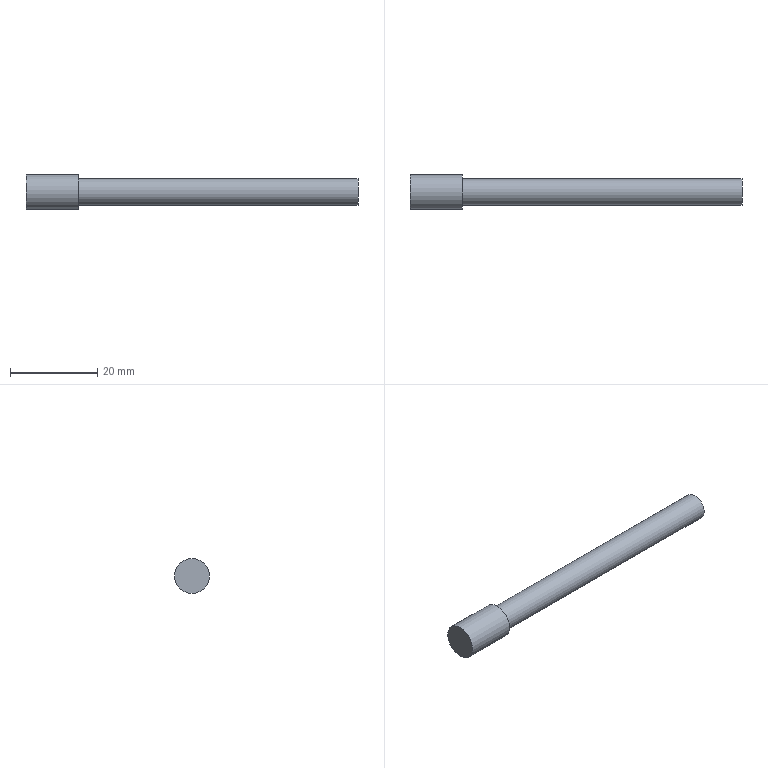Part | NX | features solid 2 | 1 solid | 5 faces | box 76 x 8 x 8 mm | volume 2413 mm3 | plane 3 | cylinder 2 | commonest cylinder face diameters 6 x1 8 x1
STEP:
#1=CARTESIAN_POINT('',(7.,-72.,-26.));
#2=VERTEX_POINT('',#1);
#3=CARTESIAN_POINT('',(7.,-72.,-23.));
#4=DIRECTION('',(1.,0.,0.));
#5=DIRECTION('',(0.,0.,-1.));
#6=AXIS2_PLACEMENT_3D('',#3,#4,#5);
#7=CIRCLE('',#6,3.);
#8=EDGE_CURVE('',#2,#2,#7,.T.);
#9=ORIENTED_EDGE('',*,*,#8,.T.);
#10=EDGE_LOOP('',(#9));
#11=FACE_BOUND('',#10,.T.);
#12=CARTESIAN_POINT('',(71.,-72.,-26.));
#13=VERTEX_POINT('',#12);
#14=CARTESIAN_POINT('',(71.,-72.,-23.));
#15=DIRECTION('',(1.,0.,0.));
#16=DIRECTION('',(0.,0.,-1.));
#17=AXIS2_PLACEMENT_3D('',#14,#15,#16);
#18=CIRCLE('',#17,3.);
#19=EDGE_CURVE('',#13,#13,#18,.T.);
#20=ORIENTED_EDGE('',*,*,#19,.F.);
#21=EDGE_LOOP('',(#20));
#22=FACE_BOUND('',#21,.T.);
#23=CARTESIAN_POINT('',(125.,-72.,-23.));
#24=DIRECTION('',(-1.,0.,0.));
#25=DIRECTION('',(0.,0.,1.));
#26=AXIS2_PLACEMENT_3D('',#23,#24,#25);
#27=CYLINDRICAL_SURFACE('',#26,3.);
#28=ADVANCED_FACE('',(#11,#22),#27,.T.);
#29=ORIENTED_EDGE('',*,*,#19,.T.);
#30=EDGE_LOOP('',(#29));
#31=FACE_BOUND('',#30,.T.);
#32=CARTESIAN_POINT('',(71.,-72.,-23.));
#33=DIRECTION('',(1.,0.,0.));
#34=DIRECTION('',(0.,0.,-1.));
#35=AXIS2_PLACEMENT_3D('',#32,#33,#34);
#36=PLANE('',#35);
#37=ADVANCED_FACE('',(#31),#36,.T.);
#38=CARTESIAN_POINT('',(7.,-72.,-27.));
#39=VERTEX_POINT('',#38);
#40=CARTESIAN_POINT('',(7.,-72.,-23.));
#41=DIRECTION('',(1.,0.,0.));
#42=DIRECTION('',(0.,0.,-1.));
#43=AXIS2_PLACEMENT_3D('',#40,#41,#42);
#44=CIRCLE('',#43,4.);
#45=EDGE_CURVE('',#39,#39,#44,.T.);
#46=ORIENTED_EDGE('',*,*,#45,.T.);
#47=EDGE_LOOP('',(#46));
#48=FACE_BOUND('',#47,.T.);
#49=ORIENTED_EDGE('',*,*,#8,.F.);
#50=EDGE_LOOP('',(#49));
#51=FACE_BOUND('',#50,.T.);
#52=CARTESIAN_POINT('',(7.,-72.,-23.));
#53=DIRECTION('',(1.,0.,0.));
#54=DIRECTION('',(0.,0.,-1.));
#55=AXIS2_PLACEMENT_3D('',#52,#53,#54);
#56=PLANE('',#55);
#57=ADVANCED_FACE('',(#48,#51),#56,.T.);
#58=ORIENTED_EDGE('',*,*,#45,.F.);
#59=EDGE_LOOP('',(#58));
#60=FACE_BOUND('',#59,.T.);
#61=CARTESIAN_POINT('',(-5.,-72.,-27.));
#62=VERTEX_POINT('',#61);
#63=CARTESIAN_POINT('',(-5.,-72.,-23.));
#64=DIRECTION('',(1.,0.,0.));
#65=DIRECTION('',(0.,0.,-1.));
#66=AXIS2_PLACEMENT_3D('',#63,#64,#65);
#67=CIRCLE('',#66,4.);
#68=EDGE_CURVE('',#62,#62,#67,.T.);
#69=ORIENTED_EDGE('',*,*,#68,.T.);
#70=EDGE_LOOP('',(#69));
#71=FACE_BOUND('',#70,.T.);
#72=CARTESIAN_POINT('',(7.,-72.,-23.));
#73=DIRECTION('',(-1.,0.,0.));
#74=DIRECTION('',(0.,0.,1.));
#75=AXIS2_PLACEMENT_3D('',#72,#73,#74);
#76=CYLINDRICAL_SURFACE('',#75,4.);
#77=ADVANCED_FACE('',(#60,#71),#76,.T.);
#78=ORIENTED_EDGE('',*,*,#68,.F.);
#79=EDGE_LOOP('',(#78));
#80=FACE_BOUND('',#79,.T.);
#81=CARTESIAN_POINT('',(-5.,-67.304,-33.));
#82=DIRECTION('',(-1.,0.,0.));
#83=DIRECTION('',(0.,0.,1.));
#84=AXIS2_PLACEMENT_3D('',#81,#82,#83);
#85=PLANE('',#84);
#86=ADVANCED_FACE('',(#80),#85,.T.);
#87=CLOSED_SHELL('',(#28,#37,#57,#77,#86));
#88=MANIFOLD_SOLID_BREP('',#87);
#89=(LENGTH_UNIT()NAMED_UNIT(*)SI_UNIT(.MILLI.,.METRE.));
#90=UNCERTAINTY_MEASURE_WITH_UNIT(LENGTH_MEASURE(0.00001),#89,'','');
#91=(NAMED_UNIT(*)PLANE_ANGLE_UNIT()SI_UNIT($,.RADIAN.));
#92=(NAMED_UNIT(*)SI_UNIT($,.STERADIAN.)SOLID_ANGLE_UNIT());
#93=(GEOMETRIC_REPRESENTATION_CONTEXT(3)GLOBAL_UNCERTAINTY_ASSIGNED_CONTEXT((#90))GLOBAL_UNIT_ASSIGNED_CONTEXT((#89,#91,#92))REPRESENTATION_CONTEXT('',''));
#94=ADVANCED_BREP_SHAPE_REPRESENTATION('',(#88),#93);